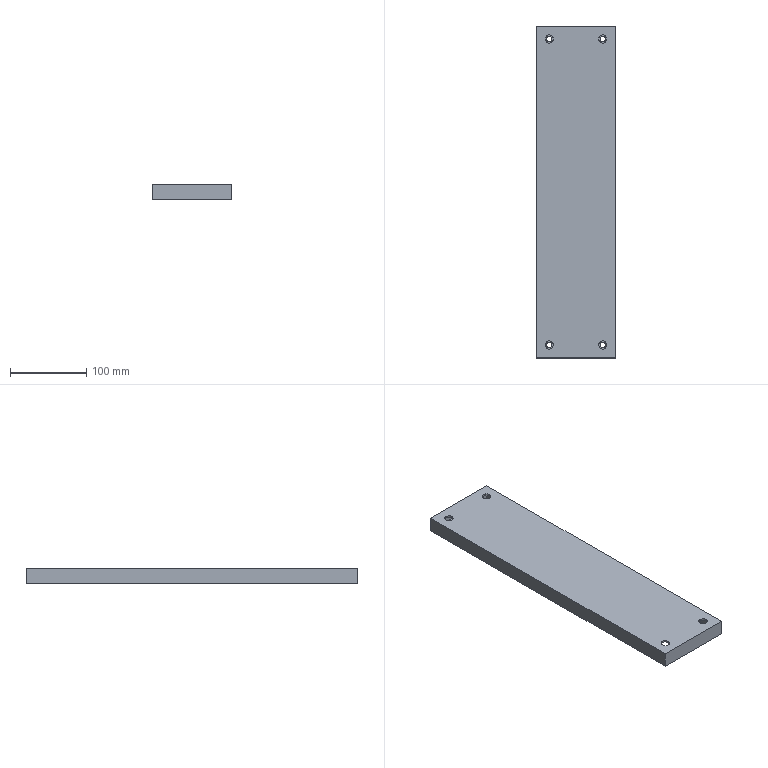Part | SolidWorks | features Extrusion 1, HoleWzd 1, ICE 1, Shell 1 | 1 solid | 32 faces | box 104 x 434 x 20 mm | volume 163254 mm3 | cylinder 16 | plane 16 | commonest cylinder face diameters 6.6 x8 11 x8
STEP:
#1=CARTESIAN_POINT('',(-29.5,200.,18.));
#2=VERTEX_POINT('',#1);
#3=CARTESIAN_POINT('',(-40.5,200.,18.));
#4=VERTEX_POINT('',#3);
#5=CARTESIAN_POINT('',(-35.,200.,18.));
#6=DIRECTION('',(0.,0.,-1.));
#7=DIRECTION('',(-1.,0.,0.));
#8=AXIS2_PLACEMENT_3D('',#5,#6,#7);
#9=CIRCLE('',#8,5.5);
#10=EDGE_CURVE('',#2,#4,#9,.T.);
#11=ORIENTED_EDGE('',*,*,#10,.T.);
#12=CARTESIAN_POINT('',(-40.5,200.,20.));
#13=VERTEX_POINT('',#12);
#14=CARTESIAN_POINT('',(-40.5,200.,20.));
#15=DIRECTION('',(0.,0.,1.));
#16=VECTOR('',#15,1000.);
#17=LINE('',#14,#16);
#18=EDGE_CURVE('',#4,#13,#17,.T.);
#19=ORIENTED_EDGE('',*,*,#18,.T.);
#20=CARTESIAN_POINT('',(-29.5,200.,20.));
#21=VERTEX_POINT('',#20);
#22=CARTESIAN_POINT('',(-35.,200.,20.));
#23=DIRECTION('',(0.,0.,1.));
#24=DIRECTION('',(1.,0.,0.));
#25=AXIS2_PLACEMENT_3D('',#22,#23,#24);
#26=CIRCLE('',#25,5.5);
#27=EDGE_CURVE('',#13,#21,#26,.T.);
#28=ORIENTED_EDGE('',*,*,#27,.T.);
#29=CARTESIAN_POINT('',(-29.5,200.,20.));
#30=DIRECTION('',(0.,0.,1.));
#31=VECTOR('',#30,1000.);
#32=LINE('',#29,#31);
#33=EDGE_CURVE('',#2,#21,#32,.T.);
#34=ORIENTED_EDGE('',*,*,#33,.F.);
#35=EDGE_LOOP('',(#11,#19,#28,#34));
#36=FACE_OUTER_BOUND('',#35,.T.);
#37=CARTESIAN_POINT('',(-35.,200.,20.));
#38=DIRECTION('',(0.,0.,1.));
#39=DIRECTION('',(1.,0.,0.));
#40=AXIS2_PLACEMENT_3D('',#37,#38,#39);
#41=CYLINDRICAL_SURFACE('',#40,5.5);
#42=ADVANCED_FACE('',(#36),#41,.F.);
#43=CARTESIAN_POINT('',(-38.3,200.,0.));
#44=VERTEX_POINT('',#43);
#45=CARTESIAN_POINT('',(-31.7,200.,0.));
#46=VERTEX_POINT('',#45);
#47=CARTESIAN_POINT('',(-35.,200.,0.));
#48=DIRECTION('',(0.,0.,1.));
#49=DIRECTION('',(1.,0.,0.));
#50=AXIS2_PLACEMENT_3D('',#47,#48,#49);
#51=CIRCLE('',#50,3.3);
#52=EDGE_CURVE('',#44,#46,#51,.T.);
#53=ORIENTED_EDGE('',*,*,#52,.F.);
#54=CARTESIAN_POINT('',(-38.3,200.,2.));
#55=VERTEX_POINT('',#54);
#56=CARTESIAN_POINT('',(-38.3,200.,20.));
#57=DIRECTION('',(0.,0.,1.));
#58=VECTOR('',#57,1000.);
#59=LINE('',#56,#58);
#60=EDGE_CURVE('',#44,#55,#59,.T.);
#61=ORIENTED_EDGE('',*,*,#60,.T.);
#62=CARTESIAN_POINT('',(-31.7,200.,2.));
#63=VERTEX_POINT('',#62);
#64=CARTESIAN_POINT('',(-35.,200.,2.));
#65=DIRECTION('',(0.,0.,-1.));
#66=DIRECTION('',(-1.,0.,0.));
#67=AXIS2_PLACEMENT_3D('',#64,#65,#66);
#68=CIRCLE('',#67,3.3);
#69=EDGE_CURVE('',#63,#55,#68,.T.);
#70=ORIENTED_EDGE('',*,*,#69,.F.);
#71=CARTESIAN_POINT('',(-31.7,200.,20.));
#72=DIRECTION('',(0.,0.,1.));
#73=VECTOR('',#72,1000.);
#74=LINE('',#71,#73);
#75=EDGE_CURVE('',#46,#63,#74,.T.);
#76=ORIENTED_EDGE('',*,*,#75,.F.);
#77=EDGE_LOOP('',(#53,#61,#70,#76));
#78=FACE_OUTER_BOUND('',#77,.T.);
#79=CARTESIAN_POINT('',(-35.,200.,20.));
#80=DIRECTION('',(0.,0.,1.));
#81=DIRECTION('',(1.,0.,0.));
#82=AXIS2_PLACEMENT_3D('',#79,#80,#81);
#83=CYLINDRICAL_SURFACE('',#82,3.3);
#84=ADVANCED_FACE('',(#78),#83,.F.);
#85=CARTESIAN_POINT('',(-29.5,-200.,18.));
#86=VERTEX_POINT('',#85);
#87=CARTESIAN_POINT('',(-40.5,-200.,18.));
#88=VERTEX_POINT('',#87);
#89=CARTESIAN_POINT('',(-35.,-200.,18.));
#90=DIRECTION('',(0.,0.,-1.));
#91=DIRECTION('',(-1.,0.,0.));
#92=AXIS2_PLACEMENT_3D('',#89,#90,#91);
#93=CIRCLE('',#92,5.5);
#94=EDGE_CURVE('',#86,#88,#93,.T.);
#95=ORIENTED_EDGE('',*,*,#94,.T.);
#96=CARTESIAN_POINT('',(-40.5,-200.,20.));
#97=VERTEX_POINT('',#96);
#98=CARTESIAN_POINT('',(-40.5,-200.,20.));
#99=DIRECTION('',(0.,0.,1.));
#100=VECTOR('',#99,1000.);
#101=LINE('',#98,#100);
#102=EDGE_CURVE('',#88,#97,#101,.T.);
#103=ORIENTED_EDGE('',*,*,#102,.T.);
#104=CARTESIAN_POINT('',(-29.5,-200.,20.));
#105=VERTEX_POINT('',#104);
#106=CARTESIAN_POINT('',(-35.,-200.,20.));
#107=DIRECTION('',(0.,0.,1.));
#108=DIRECTION('',(1.,0.,0.));
#109=AXIS2_PLACEMENT_3D('',#106,#107,#108);
#110=CIRCLE('',#109,5.5);
#111=EDGE_CURVE('',#97,#105,#110,.T.);
#112=ORIENTED_EDGE('',*,*,#111,.T.);
#113=CARTESIAN_POINT('',(-29.5,-200.,20.));
#114=DIRECTION('',(0.,0.,1.));
#115=VECTOR('',#114,1000.);
#116=LINE('',#113,#115);
#117=EDGE_CURVE('',#86,#105,#116,.T.);
#118=ORIENTED_EDGE('',*,*,#117,.F.);
#119=EDGE_LOOP('',(#95,#103,#112,#118));
#120=FACE_OUTER_BOUND('',#119,.T.);
#121=CARTESIAN_POINT('',(-35.,-200.,20.));
#122=DIRECTION('',(0.,0.,1.));
#123=DIRECTION('',(1.,0.,0.));
#124=AXIS2_PLACEMENT_3D('',#121,#122,#123);
#125=CYLINDRICAL_SURFACE('',#124,5.5);
#126=ADVANCED_FACE('',(#120),#125,.F.);
#127=CARTESIAN_POINT('',(-38.3,-200.,0.));
#128=VERTEX_POINT('',#127);
#129=CARTESIAN_POINT('',(-31.7,-200.,0.));
#130=VERTEX_POINT('',#129);
#131=CARTESIAN_POINT('',(-35.,-200.,0.));
#132=DIRECTION('',(0.,0.,1.));
#133=DIRECTION('',(1.,0.,0.));
#134=AXIS2_PLACEMENT_3D('',#131,#132,#133);
#135=CIRCLE('',#134,3.3);
#136=EDGE_CURVE('',#128,#130,#135,.T.);
#137=ORIENTED_EDGE('',*,*,#136,.F.);
#138=CARTESIAN_POINT('',(-38.3,-200.,2.));
#139=VERTEX_POINT('',#138);
#140=CARTESIAN_POINT('',(-38.3,-200.,20.));
#141=DIRECTION('',(0.,0.,1.));
#142=VECTOR('',#141,1000.);
#143=LINE('',#140,#142);
#144=EDGE_CURVE('',#128,#139,#143,.T.);
#145=ORIENTED_EDGE('',*,*,#144,.T.);
#146=CARTESIAN_POINT('',(-31.7,-200.,2.));
#147=VERTEX_POINT('',#146);
#148=CARTESIAN_POINT('',(-35.,-200.,2.));
#149=DIRECTION('',(0.,0.,-1.));
#150=DIRECTION('',(-1.,0.,0.));
#151=AXIS2_PLACEMENT_3D('',#148,#149,#150);
#152=CIRCLE('',#151,3.3);
#153=EDGE_CURVE('',#147,#139,#152,.T.);
#154=ORIENTED_EDGE('',*,*,#153,.F.);
#155=CARTESIAN_POINT('',(-31.7,-200.,20.));
#156=DIRECTION('',(0.,0.,1.));
#157=VECTOR('',#156,1000.);
#158=LINE('',#155,#157);
#159=EDGE_CURVE('',#130,#147,#158,.T.);
#160=ORIENTED_EDGE('',*,*,#159,.F.);
#161=EDGE_LOOP('',(#137,#145,#154,#160));
#162=FACE_OUTER_BOUND('',#161,.T.);
#163=CARTESIAN_POINT('',(-35.,-200.,20.));
#164=DIRECTION('',(0.,0.,1.));
#165=DIRECTION('',(1.,0.,0.));
#166=AXIS2_PLACEMENT_3D('',#163,#164,#165);
#167=CYLINDRICAL_SURFACE('',#166,3.3);
#168=ADVANCED_FACE('',(#162),#167,.F.);
#169=CARTESIAN_POINT('',(40.5,-200.,18.));
#170=VERTEX_POINT('',#169);
#171=CARTESIAN_POINT('',(29.5,-200.,18.));
#172=VERTEX_POINT('',#171);
#173=CARTESIAN_POINT('',(35.,-200.,18.));
#174=DIRECTION('',(0.,0.,-1.));
#175=DIRECTION('',(-1.,0.,0.));
#176=AXIS2_PLACEMENT_3D('',#173,#174,#175);
#177=CIRCLE('',#176,5.5);
#178=EDGE_CURVE('',#170,#172,#177,.T.);
#179=ORIENTED_EDGE('',*,*,#178,.T.);
#180=CARTESIAN_POINT('',(29.5,-200.,20.));
#181=VERTEX_POINT('',#180);
#182=CARTESIAN_POINT('',(29.5,-200.,20.));
#183=DIRECTION('',(0.,0.,1.));
#184=VECTOR('',#183,1000.);
#185=LINE('',#182,#184);
#186=EDGE_CURVE('',#172,#181,#185,.T.);
#187=ORIENTED_EDGE('',*,*,#186,.T.);
#188=CARTESIAN_POINT('',(40.5,-200.,20.));
#189=VERTEX_POINT('',#188);
#190=CARTESIAN_POINT('',(35.,-200.,20.));
#191=DIRECTION('',(0.,0.,1.));
#192=DIRECTION('',(1.,0.,0.));
#193=AXIS2_PLACEMENT_3D('',#190,#191,#192);
#194=CIRCLE('',#193,5.5);
#195=EDGE_CURVE('',#181,#189,#194,.T.);
#196=ORIENTED_EDGE('',*,*,#195,.T.);
#197=CARTESIAN_POINT('',(40.5,-200.,20.));
#198=DIRECTION('',(0.,0.,1.));
#199=VECTOR('',#198,1000.);
#200=LINE('',#197,#199);
#201=EDGE_CURVE('',#170,#189,#200,.T.);
#202=ORIENTED_EDGE('',*,*,#201,.F.);
#203=EDGE_LOOP('',(#179,#187,#196,#202));
#204=FACE_OUTER_BOUND('',#203,.T.);
#205=CARTESIAN_POINT('',(35.,-200.,20.));
#206=DIRECTION('',(0.,0.,1.));
#207=DIRECTION('',(1.,0.,0.));
#208=AXIS2_PLACEMENT_3D('',#205,#206,#207);
#209=CYLINDRICAL_SURFACE('',#208,5.5);
#210=ADVANCED_FACE('',(#204),#209,.F.);
#211=CARTESIAN_POINT('',(31.7,-200.,0.));
#212=VERTEX_POINT('',#211);
#213=CARTESIAN_POINT('',(38.3,-200.,0.));
#214=VERTEX_POINT('',#213);
#215=CARTESIAN_POINT('',(35.,-200.,0.));
#216=DIRECTION('',(0.,0.,1.));
#217=DIRECTION('',(1.,0.,0.));
#218=AXIS2_PLACEMENT_3D('',#215,#216,#217);
#219=CIRCLE('',#218,3.3);
#220=EDGE_CURVE('',#212,#214,#219,.T.);
#221=ORIENTED_EDGE('',*,*,#220,.F.);
#222=CARTESIAN_POINT('',(31.7,-200.,2.));
#223=VERTEX_POINT('',#222);
#224=CARTESIAN_POINT('',(31.7,-200.,20.));
#225=DIRECTION('',(0.,0.,1.));
#226=VECTOR('',#225,1000.);
#227=LINE('',#224,#226);
#228=EDGE_CURVE('',#212,#223,#227,.T.);
#229=ORIENTED_EDGE('',*,*,#228,.T.);
#230=CARTESIAN_POINT('',(38.3,-200.,2.));
#231=VERTEX_POINT('',#230);
#232=CARTESIAN_POINT('',(35.,-200.,2.));
#233=DIRECTION('',(0.,0.,-1.));
#234=DIRECTION('',(-1.,0.,0.));
#235=AXIS2_PLACEMENT_3D('',#232,#233,#234);
#236=CIRCLE('',#235,3.3);
#237=EDGE_CURVE('',#231,#223,#236,.T.);
#238=ORIENTED_EDGE('',*,*,#237,.F.);
#239=CARTESIAN_POINT('',(38.3,-200.,20.));
#240=DIRECTION('',(0.,0.,1.));
#241=VECTOR('',#240,1000.);
#242=LINE('',#239,#241);
#243=EDGE_CURVE('',#214,#231,#242,.T.);
#244=ORIENTED_EDGE('',*,*,#243,.F.);
#245=EDGE_LOOP('',(#221,#229,#238,#244));
#246=FACE_OUTER_BOUND('',#245,.T.);
#247=CARTESIAN_POINT('',(35.,-200.,20.));
#248=DIRECTION('',(0.,0.,1.));
#249=DIRECTION('',(1.,0.,0.));
#250=AXIS2_PLACEMENT_3D('',#247,#248,#249);
#251=CYLINDRICAL_SURFACE('',#250,3.3);
#252=ADVANCED_FACE('',(#246),#251,.F.);
#253=CARTESIAN_POINT('',(40.5,200.,18.));
#254=VERTEX_POINT('',#253);
#255=CARTESIAN_POINT('',(29.5,200.,18.));
#256=VERTEX_POINT('',#255);
#257=CARTESIAN_POINT('',(35.,200.,18.));
#258=DIRECTION('',(0.,0.,-1.));
#259=DIRECTION('',(-1.,0.,0.));
#260=AXIS2_PLACEMENT_3D('',#257,#258,#259);
#261=CIRCLE('',#260,5.5);
#262=EDGE_CURVE('',#254,#256,#261,.T.);
#263=ORIENTED_EDGE('',*,*,#262,.T.);
#264=CARTESIAN_POINT('',(29.5,200.,20.));
#265=VERTEX_POINT('',#264);
#266=CARTESIAN_POINT('',(29.5,200.,20.));
#267=DIRECTION('',(0.,0.,1.));
#268=VECTOR('',#267,1000.);
#269=LINE('',#266,#268);
#270=EDGE_CURVE('',#256,#265,#269,.T.);
#271=ORIENTED_EDGE('',*,*,#270,.T.);
#272=CARTESIAN_POINT('',(40.5,200.,20.));
#273=VERTEX_POINT('',#272);
#274=CARTESIAN_POINT('',(35.,200.,20.));
#275=DIRECTION('',(0.,0.,1.));
#276=DIRECTION('',(1.,0.,0.));
#277=AXIS2_PLACEMENT_3D('',#274,#275,#276);
#278=CIRCLE('',#277,5.5);
#279=EDGE_CURVE('',#265,#273,#278,.T.);
#280=ORIENTED_EDGE('',*,*,#279,.T.);
#281=CARTESIAN_POINT('',(40.5,200.,20.));
#282=DIRECTION('',(0.,0.,1.));
#283=VECTOR('',#282,1000.);
#284=LINE('',#281,#283);
#285=EDGE_CURVE('',#254,#273,#284,.T.);
#286=ORIENTED_EDGE('',*,*,#285,.F.);
#287=EDGE_LOOP('',(#263,#271,#280,#286));
#288=FACE_OUTER_BOUND('',#287,.T.);
#289=CARTESIAN_POINT('',(35.,200.,20.));
#290=DIRECTION('',(0.,0.,1.));
#291=DIRECTION('',(1.,0.,0.));
#292=AXIS2_PLACEMENT_3D('',#289,#290,#291);
#293=CYLINDRICAL_SURFACE('',#292,5.5);
#294=ADVANCED_FACE('',(#288),#293,.F.);
#295=CARTESIAN_POINT('',(31.7,200.,0.));
#296=VERTEX_POINT('',#295);
#297=CARTESIAN_POINT('',(38.3,200.,0.));
#298=VERTEX_POINT('',#297);
#299=CARTESIAN_POINT('',(35.,200.,0.));
#300=DIRECTION('',(0.,0.,1.));
#301=DIRECTION('',(1.,0.,0.));
#302=AXIS2_PLACEMENT_3D('',#299,#300,#301);
#303=CIRCLE('',#302,3.3);
#304=EDGE_CURVE('',#296,#298,#303,.T.);
#305=ORIENTED_EDGE('',*,*,#304,.F.);
#306=CARTESIAN_POINT('',(31.7,200.,2.));
#307=VERTEX_POINT('',#306);
#308=CARTESIAN_POINT('',(31.7,200.,20.));
#309=DIRECTION('',(0.,0.,1.));
#310=VECTOR('',#309,1000.);
#311=LINE('',#308,#310);
#312=EDGE_CURVE('',#296,#307,#311,.T.);
#313=ORIENTED_EDGE('',*,*,#312,.T.);
#314=CARTESIAN_POINT('',(38.3,200.,2.));
#315=VERTEX_POINT('',#314);
#316=CARTESIAN_POINT('',(35.,200.,2.));
#317=DIRECTION('',(0.,0.,-1.));
#318=DIRECTION('',(-1.,0.,0.));
#319=AXIS2_PLACEMENT_3D('',#316,#317,#318);
#320=CIRCLE('',#319,3.3);
#321=EDGE_CURVE('',#315,#307,#320,.T.);
#322=ORIENTED_EDGE('',*,*,#321,.F.);
#323=CARTESIAN_POINT('',(38.3,200.,20.));
#324=DIRECTION('',(0.,0.,1.));
#325=VECTOR('',#324,1000.);
#326=LINE('',#323,#325);
#327=EDGE_CURVE('',#298,#315,#326,.T.);
#328=ORIENTED_EDGE('',*,*,#327,.F.);
#329=EDGE_LOOP('',(#305,#313,#322,#328));
#330=FACE_OUTER_BOUND('',#329,.T.);
#331=CARTESIAN_POINT('',(35.,200.,20.));
#332=DIRECTION('',(0.,0.,1.));
#333=DIRECTION('',(1.,0.,0.));
#334=AXIS2_PLACEMENT_3D('',#331,#332,#333);
#335=CYLINDRICAL_SURFACE('',#334,3.3);
#336=ADVANCED_FACE('',(#330),#335,.F.);
#337=CARTESIAN_POINT('',(-35.,200.,0.));
#338=DIRECTION('',(0.,0.,1.));
#339=DIRECTION('',(1.,0.,0.));
#340=AXIS2_PLACEMENT_3D('',#337,#338,#339);
#341=CIRCLE('',#340,3.3);
#342=EDGE_CURVE('',#46,#44,#341,.T.);
#343=ORIENTED_EDGE('',*,*,#342,.T.);
#344=ORIENTED_EDGE('',*,*,#52,.T.);
#345=EDGE_LOOP('',(#343,#344));
#346=FACE_BOUND('',#345,.T.);
#347=CARTESIAN_POINT('',(-35.,-200.,0.));
#348=DIRECTION('',(0.,0.,1.));
#349=DIRECTION('',(1.,0.,0.));
#350=AXIS2_PLACEMENT_3D('',#347,#348,#349);
#351=CIRCLE('',#350,3.3);
#352=EDGE_CURVE('',#130,#128,#351,.T.);
#353=ORIENTED_EDGE('',*,*,#352,.T.);
#354=ORIENTED_EDGE('',*,*,#136,.T.);
#355=EDGE_LOOP('',(#353,#354));
#356=FACE_BOUND('',#355,.T.);
#357=CARTESIAN_POINT('',(35.,-200.,0.));
#358=DIRECTION('',(0.,0.,1.));
#359=DIRECTION('',(1.,0.,0.));
#360=AXIS2_PLACEMENT_3D('',#357,#358,#359);
#361=CIRCLE('',#360,3.3);
#362=EDGE_CURVE('',#214,#212,#361,.T.);
#363=ORIENTED_EDGE('',*,*,#362,.T.);
#364=ORIENTED_EDGE('',*,*,#220,.T.);
#365=EDGE_LOOP('',(#363,#364));
#366=FACE_BOUND('',#365,.T.);
#367=CARTESIAN_POINT('',(32.,-197.,0.));
#368=VERTEX_POINT('',#367);
#369=CARTESIAN_POINT('',(-32.,-197.,0.));
#370=VERTEX_POINT('',#369);
#371=CARTESIAN_POINT('',(32.,-197.,0.));
#372=DIRECTION('',(-1.,0.,0.));
#373=VECTOR('',#372,1000.);
#374=LINE('',#371,#373);
#375=EDGE_CURVE('',#368,#370,#374,.T.);
#376=ORIENTED_EDGE('',*,*,#375,.F.);
#377=CARTESIAN_POINT('',(32.,197.,0.));
#378=VERTEX_POINT('',#377);
#379=CARTESIAN_POINT('',(32.,-197.,0.));
#380=DIRECTION('',(0.,1.,0.));
#381=VECTOR('',#380,1000.);
#382=LINE('',#379,#381);
#383=EDGE_CURVE('',#368,#378,#382,.T.);
#384=ORIENTED_EDGE('',*,*,#383,.T.);
#385=CARTESIAN_POINT('',(-32.,197.,0.));
#386=VERTEX_POINT('',#385);
#387=CARTESIAN_POINT('',(32.,197.,0.));
#388=DIRECTION('',(-1.,0.,0.));
#389=VECTOR('',#388,1000.);
#390=LINE('',#387,#389);
#391=EDGE_CURVE('',#378,#386,#390,.T.);
#392=ORIENTED_EDGE('',*,*,#391,.T.);
#393=CARTESIAN_POINT('',(-32.,-197.,0.));
#394=DIRECTION('',(0.,1.,0.));
#395=VECTOR('',#394,1000.);
#396=LINE('',#393,#395);
#397=EDGE_CURVE('',#370,#386,#396,.T.);
#398=ORIENTED_EDGE('',*,*,#397,.F.);
#399=EDGE_LOOP('',(#376,#384,#392,#398));
#400=FACE_BOUND('',#399,.T.);
#401=CARTESIAN_POINT('',(52.,-217.,0.));
#402=VERTEX_POINT('',#401);
#403=CARTESIAN_POINT('',(52.,217.,0.));
#404=VERTEX_POINT('',#403);
#405=CARTESIAN_POINT('',(52.,-217.,0.));
#406=DIRECTION('',(0.,1.,0.));
#407=VECTOR('',#406,1000.);
#408=LINE('',#405,#407);
#409=EDGE_CURVE('',#402,#404,#408,.T.);
#410=ORIENTED_EDGE('',*,*,#409,.F.);
#411=CARTESIAN_POINT('',(-52.,-217.,0.));
#412=VERTEX_POINT('',#411);
#413=CARTESIAN_POINT('',(-52.,-217.,0.));
#414=DIRECTION('',(1.,0.,0.));
#415=VECTOR('',#414,1000.);
#416=LINE('',#413,#415);
#417=EDGE_CURVE('',#412,#402,#416,.T.);
#418=ORIENTED_EDGE('',*,*,#417,.F.);
#419=CARTESIAN_POINT('',(-52.,217.,0.));
#420=VERTEX_POINT('',#419);
#421=CARTESIAN_POINT('',(-52.,-217.,0.));
#422=DIRECTION('',(0.,-1.,0.));
#423=VECTOR('',#422,1000.);
#424=LINE('',#421,#423);
#425=EDGE_CURVE('',#420,#412,#424,.T.);
#426=ORIENTED_EDGE('',*,*,#425,.F.);
#427=CARTESIAN_POINT('',(-52.,217.,0.));
#428=DIRECTION('',(-1.,0.,0.));
#429=VECTOR('',#428,1000.);
#430=LINE('',#427,#429);
#431=EDGE_CURVE('',#404,#420,#430,.T.);
#432=ORIENTED_EDGE('',*,*,#431,.F.);
#433=EDGE_LOOP('',(#410,#418,#426,#432));
#434=FACE_OUTER_BOUND('',#433,.T.);
#435=CARTESIAN_POINT('',(35.,200.,0.));
#436=DIRECTION('',(0.,0.,1.));
#437=DIRECTION('',(1.,0.,0.));
#438=AXIS2_PLACEMENT_3D('',#435,#436,#437);
#439=CIRCLE('',#438,3.3);
#440=EDGE_CURVE('',#298,#296,#439,.T.);
#441=ORIENTED_EDGE('',*,*,#440,.T.);
#442=ORIENTED_EDGE('',*,*,#304,.T.);
#443=EDGE_LOOP('',(#441,#442));
#444=FACE_BOUND('',#443,.T.);
#445=CARTESIAN_POINT('',(0.,0.,0.));
#446=DIRECTION('',(0.,0.,-1.));
#447=DIRECTION('',(-1.,0.,0.));
#448=AXIS2_PLACEMENT_3D('',#445,#446,#447);
#449=PLANE('',#448);
#450=ADVANCED_FACE('',(#346,#356,#366,#400,#434,#444),#449,.T.);
#451=ORIENTED_EDGE('',*,*,#409,.T.);
#452=CARTESIAN_POINT('',(52.,217.,20.));
#453=VERTEX_POINT('',#452);
#454=CARTESIAN_POINT('',(52.,217.,20.));
#455=DIRECTION('',(0.,0.,-1.));
#456=VECTOR('',#455,1000.);
#457=LINE('',#454,#456);
#458=EDGE_CURVE('',#453,#404,#457,.T.);
#459=ORIENTED_EDGE('',*,*,#458,.F.);
#460=CARTESIAN_POINT('',(52.,-217.,20.));
#461=VERTEX_POINT('',#460);
#462=CARTESIAN_POINT('',(52.,-217.,20.));
#463=DIRECTION('',(0.,1.,0.));
#464=VECTOR('',#463,1000.);
#465=LINE('',#462,#464);
#466=EDGE_CURVE('',#461,#453,#465,.T.);
#467=ORIENTED_EDGE('',*,*,#466,.F.);
#468=CARTESIAN_POINT('',(52.,-217.,20.));
#469=DIRECTION('',(0.,0.,-1.));
#470=VECTOR('',#469,1000.);
#471=LINE('',#468,#470);
#472=EDGE_CURVE('',#461,#402,#471,.T.);
#473=ORIENTED_EDGE('',*,*,#472,.T.);
#474=EDGE_LOOP('',(#451,#459,#467,#473));
#475=FACE_OUTER_BOUND('',#474,.T.);
#476=CARTESIAN_POINT('',(52.,-217.,20.));
#477=DIRECTION('',(-1.,0.,0.));
#478=DIRECTION('',(0.,0.,1.));
#479=AXIS2_PLACEMENT_3D('',#476,#477,#478);
#480=PLANE('',#479);
#481=ADVANCED_FACE('',(#475),#480,.F.);
#482=ORIENTED_EDGE('',*,*,#431,.T.);
#483=CARTESIAN_POINT('',(-52.,217.,20.));
#484=VERTEX_POINT('',#483);
#485=CARTESIAN_POINT('',(-52.,217.,20.));
#486=DIRECTION('',(0.,0.,-1.));
#487=VECTOR('',#486,1000.);
#488=LINE('',#485,#487);
#489=EDGE_CURVE('',#484,#420,#488,.T.);
#490=ORIENTED_EDGE('',*,*,#489,.F.);
#491=CARTESIAN_POINT('',(-52.,217.,20.));
#492=DIRECTION('',(-1.,0.,0.));
#493=VECTOR('',#492,1000.);
#494=LINE('',#491,#493);
#495=EDGE_CURVE('',#453,#484,#494,.T.);
#496=ORIENTED_EDGE('',*,*,#495,.F.);
#497=ORIENTED_EDGE('',*,*,#458,.T.);
#498=EDGE_LOOP('',(#482,#490,#496,#497));
#499=FACE_OUTER_BOUND('',#498,.T.);
#500=CARTESIAN_POINT('',(-52.,217.,20.));
#501=DIRECTION('',(0.,-1.,0.));
#502=DIRECTION('',(0.,0.,-1.));
#503=AXIS2_PLACEMENT_3D('',#500,#501,#502);
#504=PLANE('',#503);
#505=ADVANCED_FACE('',(#499),#504,.F.);
#506=ORIENTED_EDGE('',*,*,#425,.T.);
#507=CARTESIAN_POINT('',(-52.,-217.,20.));
#508=VERTEX_POINT('',#507);
#509=CARTESIAN_POINT('',(-52.,-217.,20.));
#510=DIRECTION('',(0.,0.,-1.));
#511=VECTOR('',#510,1000.);
#512=LINE('',#509,#511);
#513=EDGE_CURVE('',#508,#412,#512,.T.);
#514=ORIENTED_EDGE('',*,*,#513,.F.);
#515=CARTESIAN_POINT('',(-52.,-217.,20.));
#516=DIRECTION('',(0.,-1.,0.));
#517=VECTOR('',#516,1000.);
#518=LINE('',#515,#517);
#519=EDGE_CURVE('',#484,#508,#518,.T.);
#520=ORIENTED_EDGE('',*,*,#519,.F.);
#521=ORIENTED_EDGE('',*,*,#489,.T.);
#522=EDGE_LOOP('',(#506,#514,#520,#521));
#523=FACE_OUTER_BOUND('',#522,.T.);
#524=CARTESIAN_POINT('',(-52.,-217.,20.));
#525=DIRECTION('',(1.,0.,0.));
#526=DIRECTION('',(0.,0.,-1.));
#527=AXIS2_PLACEMENT_3D('',#524,#525,#526);
#528=PLANE('',#527);
#529=ADVANCED_FACE('',(#523),#528,.F.);
#530=ORIENTED_EDGE('',*,*,#417,.T.);
#531=ORIENTED_EDGE('',*,*,#472,.F.);
#532=CARTESIAN_POINT('',(-52.,-217.,20.));
#533=DIRECTION('',(1.,0.,0.));
#534=VECTOR('',#533,1000.);
#535=LINE('',#532,#534);
#536=EDGE_CURVE('',#508,#461,#535,.T.);
#537=ORIENTED_EDGE('',*,*,#536,.F.);
#538=ORIENTED_EDGE('',*,*,#513,.T.);
#539=EDGE_LOOP('',(#530,#531,#537,#538));
#540=FACE_OUTER_BOUND('',#539,.T.);
#541=CARTESIAN_POINT('',(-52.,-217.,20.));
#542=DIRECTION('',(0.,1.,0.));
#543=DIRECTION('',(0.,0.,1.));
#544=AXIS2_PLACEMENT_3D('',#541,#542,#543);
#545=PLANE('',#544);
#546=ADVANCED_FACE('',(#540),#545,.F.);
#547=CARTESIAN_POINT('',(-35.,200.,20.));
#548=DIRECTION('',(0.,0.,1.));
#549=DIRECTION('',(1.,0.,0.));
#550=AXIS2_PLACEMENT_3D('',#547,#548,#549);
#551=CIRCLE('',#550,5.5);
#552=EDGE_CURVE('',#21,#13,#551,.T.);
#553=ORIENTED_EDGE('',*,*,#552,.F.);
#554=ORIENTED_EDGE('',*,*,#27,.F.);
#555=EDGE_LOOP('',(#553,#554));
#556=FACE_BOUND('',#555,.T.);
#557=CARTESIAN_POINT('',(-35.,-200.,20.));
#558=DIRECTION('',(0.,0.,1.));
#559=DIRECTION('',(1.,0.,0.));
#560=AXIS2_PLACEMENT_3D('',#557,#558,#559);
#561=CIRCLE('',#560,5.5);
#562=EDGE_CURVE('',#105,#97,#561,.T.);
#563=ORIENTED_EDGE('',*,*,#562,.F.);
#564=ORIENTED_EDGE('',*,*,#111,.F.);
#565=EDGE_LOOP('',(#563,#564));
#566=FACE_BOUND('',#565,.T.);
#567=CARTESIAN_POINT('',(35.,-200.,20.));
#568=DIRECTION('',(0.,0.,1.));
#569=DIRECTION('',(1.,0.,0.));
#570=AXIS2_PLACEMENT_3D('',#567,#568,#569);
#571=CIRCLE('',#570,5.5);
#572=EDGE_CURVE('',#189,#181,#571,.T.);
#573=ORIENTED_EDGE('',*,*,#572,.F.);
#574=ORIENTED_EDGE('',*,*,#195,.F.);
#575=EDGE_LOOP('',(#573,#574));
#576=FACE_BOUND('',#575,.T.);
#577=CARTESIAN_POINT('',(35.,200.,20.));
#578=DIRECTION('',(0.,0.,1.));
#579=DIRECTION('',(1.,0.,0.));
#580=AXIS2_PLACEMENT_3D('',#577,#578,#579);
#581=CIRCLE('',#580,5.5);
#582=EDGE_CURVE('',#273,#265,#581,.T.);
#583=ORIENTED_EDGE('',*,*,#582,.F.);
#584=ORIENTED_EDGE('',*,*,#279,.F.);
#585=EDGE_LOOP('',(#583,#584));
#586=FACE_BOUND('',#585,.T.);
#587=ORIENTED_EDGE('',*,*,#466,.T.);
#588=ORIENTED_EDGE('',*,*,#495,.T.);
#589=ORIENTED_EDGE('',*,*,#519,.T.);
#590=ORIENTED_EDGE('',*,*,#536,.T.);
#591=EDGE_LOOP('',(#587,#588,#589,#590));
#592=FACE_OUTER_BOUND('',#591,.T.);
#593=CARTESIAN_POINT('',(0.,0.,20.));
#594=DIRECTION('',(0.,0.,-1.));
#595=DIRECTION('',(-1.,0.,0.));
#596=AXIS2_PLACEMENT_3D('',#593,#594,#595);
#597=PLANE('',#596);
#598=ADVANCED_FACE('',(#556,#566,#576,#586,#592),#597,.F.);
#599=ORIENTED_EDGE('',*,*,#383,.F.);
#600=CARTESIAN_POINT('',(32.,-197.,2.));
#601=VERTEX_POINT('',#600);
#602=CARTESIAN_POINT('',(32.,-197.,2.));
#603=DIRECTION('',(0.,0.,-1.));
#604=VECTOR('',#603,1000.);
#605=LINE('',#602,#604);
#606=EDGE_CURVE('',#601,#368,#605,.T.);
#607=ORIENTED_EDGE('',*,*,#606,.F.);
#608=CARTESIAN_POINT('',(32.,197.,2.));
#609=VERTEX_POINT('',#608);
#610=CARTESIAN_POINT('',(32.,-197.,2.));
#611=DIRECTION('',(0.,1.,0.));
#612=VECTOR('',#611,1000.);
#613=LINE('',#610,#612);
#614=EDGE_CURVE('',#601,#609,#613,.T.);
#615=ORIENTED_EDGE('',*,*,#614,.T.);
#616=CARTESIAN_POINT('',(32.,197.,2.));
#617=DIRECTION('',(0.,0.,-1.));
#618=VECTOR('',#617,1000.);
#619=LINE('',#616,#618);
#620=EDGE_CURVE('',#609,#378,#619,.T.);
#621=ORIENTED_EDGE('',*,*,#620,.T.);
#622=EDGE_LOOP('',(#599,#607,#615,#621));
#623=FACE_OUTER_BOUND('',#622,.T.);
#624=CARTESIAN_POINT('',(32.,-197.,2.));
#625=DIRECTION('',(-1.,0.,0.));
#626=DIRECTION('',(0.,0.,1.));
#627=AXIS2_PLACEMENT_3D('',#624,#625,#626);
#628=PLANE('',#627);
#629=ADVANCED_FACE('',(#623),#628,.T.);
#630=ORIENTED_EDGE('',*,*,#391,.F.);
#631=ORIENTED_EDGE('',*,*,#620,.F.);
#632=CARTESIAN_POINT('',(-32.,197.,2.));
#633=VERTEX_POINT('',#632);
#634=CARTESIAN_POINT('',(32.,197.,2.));
#635=DIRECTION('',(-1.,0.,0.));
#636=VECTOR('',#635,1000.);
#637=LINE('',#634,#636);
#638=EDGE_CURVE('',#609,#633,#637,.T.);
#639=ORIENTED_EDGE('',*,*,#638,.T.);
#640=CARTESIAN_POINT('',(-32.,197.,2.));
#641=DIRECTION('',(0.,0.,-1.));
#642=VECTOR('',#641,1000.);
#643=LINE('',#640,#642);
#644=EDGE_CURVE('',#633,#386,#643,.T.);
#645=ORIENTED_EDGE('',*,*,#644,.T.);
#646=EDGE_LOOP('',(#630,#631,#639,#645));
#647=FACE_OUTER_BOUND('',#646,.T.);
#648=CARTESIAN_POINT('',(32.,197.,2.));
#649=DIRECTION('',(0.,-1.,0.));
#650=DIRECTION('',(0.,0.,-1.));
#651=AXIS2_PLACEMENT_3D('',#648,#649,#650);
#652=PLANE('',#651);
#653=ADVANCED_FACE('',(#647),#652,.T.);
#654=ORIENTED_EDGE('',*,*,#397,.T.);
#655=ORIENTED_EDGE('',*,*,#644,.F.);
#656=CARTESIAN_POINT('',(-32.,-197.,2.));
#657=VERTEX_POINT('',#656);
#658=CARTESIAN_POINT('',(-32.,-197.,2.));
#659=DIRECTION('',(0.,1.,0.));
#660=VECTOR('',#659,1000.);
#661=LINE('',#658,#660);
#662=EDGE_CURVE('',#657,#633,#661,.T.);
#663=ORIENTED_EDGE('',*,*,#662,.F.);
#664=CARTESIAN_POINT('',(-32.,-197.,2.));
#665=DIRECTION('',(0.,0.,-1.));
#666=VECTOR('',#665,1000.);
#667=LINE('',#664,#666);
#668=EDGE_CURVE('',#657,#370,#667,.T.);
#669=ORIENTED_EDGE('',*,*,#668,.T.);
#670=EDGE_LOOP('',(#654,#655,#663,#669));
#671=FACE_OUTER_BOUND('',#670,.T.);
#672=CARTESIAN_POINT('',(-32.,-197.,2.));
#673=DIRECTION('',(-1.,0.,0.));
#674=DIRECTION('',(0.,0.,1.));
#675=AXIS2_PLACEMENT_3D('',#672,#673,#674);
#676=PLANE('',#675);
#677=ADVANCED_FACE('',(#671),#676,.F.);
#678=ORIENTED_EDGE('',*,*,#375,.T.);
#679=ORIENTED_EDGE('',*,*,#668,.F.);
#680=CARTESIAN_POINT('',(32.,-197.,2.));
#681=DIRECTION('',(-1.,0.,0.));
#682=VECTOR('',#681,1000.);
#683=LINE('',#680,#682);
#684=EDGE_CURVE('',#601,#657,#683,.T.);
#685=ORIENTED_EDGE('',*,*,#684,.F.);
#686=ORIENTED_EDGE('',*,*,#606,.T.);
#687=EDGE_LOOP('',(#678,#679,#685,#686));
#688=FACE_OUTER_BOUND('',#687,.T.);
#689=CARTESIAN_POINT('',(32.,-197.,2.));
#690=DIRECTION('',(0.,-1.,0.));
#691=DIRECTION('',(0.,0.,-1.));
#692=AXIS2_PLACEMENT_3D('',#689,#690,#691);
#693=PLANE('',#692);
#694=ADVANCED_FACE('',(#688),#693,.F.);
#695=ORIENTED_EDGE('',*,*,#69,.T.);
#696=CARTESIAN_POINT('',(-35.,200.,2.));
#697=DIRECTION('',(0.,0.,-1.));
#698=DIRECTION('',(-1.,0.,0.));
#699=AXIS2_PLACEMENT_3D('',#696,#697,#698);
#700=CIRCLE('',#699,3.3);
#701=EDGE_CURVE('',#55,#63,#700,.T.);
#702=ORIENTED_EDGE('',*,*,#701,.T.);
#703=EDGE_LOOP('',(#695,#702));
#704=FACE_BOUND('',#703,.T.);
#705=ORIENTED_EDGE('',*,*,#153,.T.);
#706=CARTESIAN_POINT('',(-35.,-200.,2.));
#707=DIRECTION('',(0.,0.,-1.));
#708=DIRECTION('',(-1.,0.,0.));
#709=AXIS2_PLACEMENT_3D('',#706,#707,#708);
#710=CIRCLE('',#709,3.3);
#711=EDGE_CURVE('',#139,#147,#710,.T.);
#712=ORIENTED_EDGE('',*,*,#711,.T.);
#713=EDGE_LOOP('',(#705,#712));
#714=FACE_BOUND('',#713,.T.);
#715=ORIENTED_EDGE('',*,*,#237,.T.);
#716=CARTESIAN_POINT('',(35.,-200.,2.));
#717=DIRECTION('',(0.,0.,-1.));
#718=DIRECTION('',(-1.,0.,0.));
#719=AXIS2_PLACEMENT_3D('',#716,#717,#718);
#720=CIRCLE('',#719,3.3);
#721=EDGE_CURVE('',#223,#231,#720,.T.);
#722=ORIENTED_EDGE('',*,*,#721,.T.);
#723=EDGE_LOOP('',(#715,#722));
#724=FACE_BOUND('',#723,.T.);
#725=ORIENTED_EDGE('',*,*,#321,.T.);
#726=CARTESIAN_POINT('',(35.,200.,2.));
#727=DIRECTION('',(0.,0.,-1.));
#728=DIRECTION('',(-1.,0.,0.));
#729=AXIS2_PLACEMENT_3D('',#726,#727,#728);
#730=CIRCLE('',#729,3.3);
#731=EDGE_CURVE('',#307,#315,#730,.T.);
#732=ORIENTED_EDGE('',*,*,#731,.T.);
#733=EDGE_LOOP('',(#725,#732));
#734=FACE_BOUND('',#733,.T.);
#735=CARTESIAN_POINT('',(50.,-215.,2.));
#736=VERTEX_POINT('',#735);
#737=CARTESIAN_POINT('',(50.,215.,2.));
#738=VERTEX_POINT('',#737);
#739=CARTESIAN_POINT('',(50.,0.,2.));
#740=DIRECTION('',(0.,1.,0.));
#741=VECTOR('',#740,1000.);
#742=LINE('',#739,#741);
#743=EDGE_CURVE('',#736,#738,#742,.T.);
#744=ORIENTED_EDGE('',*,*,#743,.T.);
#745=CARTESIAN_POINT('',(-50.,215.,2.));
#746=VERTEX_POINT('',#745);
#747=CARTESIAN_POINT('',(0.,215.,2.));
#748=DIRECTION('',(-1.,0.,0.));
#749=VECTOR('',#748,1000.);
#750=LINE('',#747,#749);
#751=EDGE_CURVE('',#738,#746,#750,.T.);
#752=ORIENTED_EDGE('',*,*,#751,.T.);
#753=CARTESIAN_POINT('',(-50.,-215.,2.));
#754=VERTEX_POINT('',#753);
#755=CARTESIAN_POINT('',(-50.,0.,2.));
#756=DIRECTION('',(0.,-1.,0.));
#757=VECTOR('',#756,1000.);
#758=LINE('',#755,#757);
#759=EDGE_CURVE('',#746,#754,#758,.T.);
#760=ORIENTED_EDGE('',*,*,#759,.T.);
#761=CARTESIAN_POINT('',(0.,-215.,2.));
#762=DIRECTION('',(1.,0.,0.));
#763=VECTOR('',#762,1000.);
#764=LINE('',#761,#763);
#765=EDGE_CURVE('',#754,#736,#764,.T.);
#766=ORIENTED_EDGE('',*,*,#765,.T.);
#767=EDGE_LOOP('',(#744,#752,#760,#766));
#768=FACE_OUTER_BOUND('',#767,.T.);
#769=ORIENTED_EDGE('',*,*,#684,.T.);
#770=ORIENTED_EDGE('',*,*,#662,.T.);
#771=ORIENTED_EDGE('',*,*,#638,.F.);
#772=ORIENTED_EDGE('',*,*,#614,.F.);
#773=EDGE_LOOP('',(#769,#770,#771,#772));
#774=FACE_BOUND('',#773,.T.);
#775=CARTESIAN_POINT('',(0.,0.,2.));
#776=DIRECTION('',(0.,0.,-1.));
#777=DIRECTION('',(-1.,0.,0.));
#778=AXIS2_PLACEMENT_3D('',#775,#776,#777);
#779=PLANE('',#778);
#780=ADVANCED_FACE('',(#704,#714,#724,#734,#768,#774),#779,.F.);
#781=ORIENTED_EDGE('',*,*,#743,.F.);
#782=CARTESIAN_POINT('',(50.,-215.,18.));
#783=VERTEX_POINT('',#782);
#784=CARTESIAN_POINT('',(50.,-215.,20.));
#785=DIRECTION('',(0.,0.,-1.));
#786=VECTOR('',#785,1000.);
#787=LINE('',#784,#786);
#788=EDGE_CURVE('',#783,#736,#787,.T.);
#789=ORIENTED_EDGE('',*,*,#788,.F.);
#790=CARTESIAN_POINT('',(50.,215.,18.));
#791=VERTEX_POINT('',#790);
#792=CARTESIAN_POINT('',(50.,0.,18.));
#793=DIRECTION('',(0.,1.,0.));
#794=VECTOR('',#793,1000.);
#795=LINE('',#792,#794);
#796=EDGE_CURVE('',#783,#791,#795,.T.);
#797=ORIENTED_EDGE('',*,*,#796,.T.);
#798=CARTESIAN_POINT('',(50.,215.,20.));
#799=DIRECTION('',(0.,0.,-1.));
#800=VECTOR('',#799,1000.);
#801=LINE('',#798,#800);
#802=EDGE_CURVE('',#791,#738,#801,.T.);
#803=ORIENTED_EDGE('',*,*,#802,.T.);
#804=EDGE_LOOP('',(#781,#789,#797,#803));
#805=FACE_OUTER_BOUND('',#804,.T.);
#806=CARTESIAN_POINT('',(50.,-217.,20.));
#807=DIRECTION('',(-1.,0.,0.));
#808=DIRECTION('',(0.,0.,1.));
#809=AXIS2_PLACEMENT_3D('',#806,#807,#808);
#810=PLANE('',#809);
#811=ADVANCED_FACE('',(#805),#810,.T.);
#812=ORIENTED_EDGE('',*,*,#751,.F.);
#813=ORIENTED_EDGE('',*,*,#802,.F.);
#814=CARTESIAN_POINT('',(-50.,215.,18.));
#815=VERTEX_POINT('',#814);
#816=CARTESIAN_POINT('',(0.,215.,18.));
#817=DIRECTION('',(-1.,0.,0.));
#818=VECTOR('',#817,1000.);
#819=LINE('',#816,#818);
#820=EDGE_CURVE('',#791,#815,#819,.T.);
#821=ORIENTED_EDGE('',*,*,#820,.T.);
#822=CARTESIAN_POINT('',(-50.,215.,20.));
#823=DIRECTION('',(0.,0.,-1.));
#824=VECTOR('',#823,1000.);
#825=LINE('',#822,#824);
#826=EDGE_CURVE('',#815,#746,#825,.T.);
#827=ORIENTED_EDGE('',*,*,#826,.T.);
#828=EDGE_LOOP('',(#812,#813,#821,#827));
#829=FACE_OUTER_BOUND('',#828,.T.);
#830=CARTESIAN_POINT('',(-52.,215.,20.));
#831=DIRECTION('',(0.,-1.,0.));
#832=DIRECTION('',(0.,0.,-1.));
#833=AXIS2_PLACEMENT_3D('',#830,#831,#832);
#834=PLANE('',#833);
#835=ADVANCED_FACE('',(#829),#834,.T.);
#836=ORIENTED_EDGE('',*,*,#759,.F.);
#837=ORIENTED_EDGE('',*,*,#826,.F.);
#838=CARTESIAN_POINT('',(-50.,-215.,18.));
#839=VERTEX_POINT('',#838);
#840=CARTESIAN_POINT('',(-50.,0.,18.));
#841=DIRECTION('',(0.,-1.,0.));
#842=VECTOR('',#841,1000.);
#843=LINE('',#840,#842);
#844=EDGE_CURVE('',#815,#839,#843,.T.);
#845=ORIENTED_EDGE('',*,*,#844,.T.);
#846=CARTESIAN_POINT('',(-50.,-215.,20.));
#847=DIRECTION('',(0.,0.,-1.));
#848=VECTOR('',#847,1000.);
#849=LINE('',#846,#848);
#850=EDGE_CURVE('',#839,#754,#849,.T.);
#851=ORIENTED_EDGE('',*,*,#850,.T.);
#852=EDGE_LOOP('',(#836,#837,#845,#851));
#853=FACE_OUTER_BOUND('',#852,.T.);
#854=CARTESIAN_POINT('',(-50.,-217.,20.));
#855=DIRECTION('',(1.,0.,0.));
#856=DIRECTION('',(0.,0.,-1.));
#857=AXIS2_PLACEMENT_3D('',#854,#855,#856);
#858=PLANE('',#857);
#859=ADVANCED_FACE('',(#853),#858,.T.);
#860=ORIENTED_EDGE('',*,*,#765,.F.);
#861=ORIENTED_EDGE('',*,*,#850,.F.);
#862=CARTESIAN_POINT('',(0.,-215.,18.));
#863=DIRECTION('',(1.,0.,0.));
#864=VECTOR('',#863,1000.);
#865=LINE('',#862,#864);
#866=EDGE_CURVE('',#839,#783,#865,.T.);
#867=ORIENTED_EDGE('',*,*,#866,.T.);
#868=ORIENTED_EDGE('',*,*,#788,.T.);
#869=EDGE_LOOP('',(#860,#861,#867,#868));
#870=FACE_OUTER_BOUND('',#869,.T.);
#871=CARTESIAN_POINT('',(-52.,-215.,20.));
#872=DIRECTION('',(0.,1.,0.));
#873=DIRECTION('',(0.,0.,1.));
#874=AXIS2_PLACEMENT_3D('',#871,#872,#873);
#875=PLANE('',#874);
#876=ADVANCED_FACE('',(#870),#875,.T.);
#877=ORIENTED_EDGE('',*,*,#10,.F.);
#878=CARTESIAN_POINT('',(-35.,200.,18.));
#879=DIRECTION('',(0.,0.,-1.));
#880=DIRECTION('',(-1.,0.,0.));
#881=AXIS2_PLACEMENT_3D('',#878,#879,#880);
#882=CIRCLE('',#881,5.5);
#883=EDGE_CURVE('',#4,#2,#882,.T.);
#884=ORIENTED_EDGE('',*,*,#883,.F.);
#885=EDGE_LOOP('',(#877,#884));
#886=FACE_BOUND('',#885,.T.);
#887=ORIENTED_EDGE('',*,*,#94,.F.);
#888=CARTESIAN_POINT('',(-35.,-200.,18.));
#889=DIRECTION('',(0.,0.,-1.));
#890=DIRECTION('',(-1.,0.,0.));
#891=AXIS2_PLACEMENT_3D('',#888,#889,#890);
#892=CIRCLE('',#891,5.5);
#893=EDGE_CURVE('',#88,#86,#892,.T.);
#894=ORIENTED_EDGE('',*,*,#893,.F.);
#895=EDGE_LOOP('',(#887,#894));
#896=FACE_BOUND('',#895,.T.);
#897=ORIENTED_EDGE('',*,*,#178,.F.);
#898=CARTESIAN_POINT('',(35.,-200.,18.));
#899=DIRECTION('',(0.,0.,-1.));
#900=DIRECTION('',(-1.,0.,0.));
#901=AXIS2_PLACEMENT_3D('',#898,#899,#900);
#902=CIRCLE('',#901,5.5);
#903=EDGE_CURVE('',#172,#170,#902,.T.);
#904=ORIENTED_EDGE('',*,*,#903,.F.);
#905=EDGE_LOOP('',(#897,#904));
#906=FACE_BOUND('',#905,.T.);
#907=ORIENTED_EDGE('',*,*,#262,.F.);
#908=CARTESIAN_POINT('',(35.,200.,18.));
#909=DIRECTION('',(0.,0.,-1.));
#910=DIRECTION('',(-1.,0.,0.));
#911=AXIS2_PLACEMENT_3D('',#908,#909,#910);
#912=CIRCLE('',#911,5.5);
#913=EDGE_CURVE('',#256,#254,#912,.T.);
#914=ORIENTED_EDGE('',*,*,#913,.F.);
#915=EDGE_LOOP('',(#907,#914));
#916=FACE_BOUND('',#915,.T.);
#917=ORIENTED_EDGE('',*,*,#796,.F.);
#918=ORIENTED_EDGE('',*,*,#866,.F.);
#919=ORIENTED_EDGE('',*,*,#844,.F.);
#920=ORIENTED_EDGE('',*,*,#820,.F.);
#921=EDGE_LOOP('',(#917,#918,#919,#920));
#922=FACE_OUTER_BOUND('',#921,.T.);
#923=CARTESIAN_POINT('',(0.,0.,18.));
#924=DIRECTION('',(0.,0.,-1.));
#925=DIRECTION('',(-1.,0.,0.));
#926=AXIS2_PLACEMENT_3D('',#923,#924,#925);
#927=PLANE('',#926);
#928=ADVANCED_FACE('',(#886,#896,#906,#916,#922),#927,.T.);
#929=ORIENTED_EDGE('',*,*,#312,.F.);
#930=ORIENTED_EDGE('',*,*,#440,.F.);
#931=ORIENTED_EDGE('',*,*,#327,.T.);
#932=ORIENTED_EDGE('',*,*,#731,.F.);
#933=EDGE_LOOP('',(#929,#930,#931,#932));
#934=FACE_OUTER_BOUND('',#933,.T.);
#935=CARTESIAN_POINT('',(35.,200.,20.));
#936=DIRECTION('',(0.,0.,1.));
#937=DIRECTION('',(1.,0.,0.));
#938=AXIS2_PLACEMENT_3D('',#935,#936,#937);
#939=CYLINDRICAL_SURFACE('',#938,3.3);
#940=ADVANCED_FACE('',(#934),#939,.F.);
#941=ORIENTED_EDGE('',*,*,#270,.F.);
#942=ORIENTED_EDGE('',*,*,#913,.T.);
#943=ORIENTED_EDGE('',*,*,#285,.T.);
#944=ORIENTED_EDGE('',*,*,#582,.T.);
#945=EDGE_LOOP('',(#941,#942,#943,#944));
#946=FACE_OUTER_BOUND('',#945,.T.);
#947=CARTESIAN_POINT('',(35.,200.,20.));
#948=DIRECTION('',(0.,0.,1.));
#949=DIRECTION('',(1.,0.,0.));
#950=AXIS2_PLACEMENT_3D('',#947,#948,#949);
#951=CYLINDRICAL_SURFACE('',#950,5.5);
#952=ADVANCED_FACE('',(#946),#951,.F.);
#953=ORIENTED_EDGE('',*,*,#228,.F.);
#954=ORIENTED_EDGE('',*,*,#362,.F.);
#955=ORIENTED_EDGE('',*,*,#243,.T.);
#956=ORIENTED_EDGE('',*,*,#721,.F.);
#957=EDGE_LOOP('',(#953,#954,#955,#956));
#958=FACE_OUTER_BOUND('',#957,.T.);
#959=CARTESIAN_POINT('',(35.,-200.,20.));
#960=DIRECTION('',(0.,0.,1.));
#961=DIRECTION('',(1.,0.,0.));
#962=AXIS2_PLACEMENT_3D('',#959,#960,#961);
#963=CYLINDRICAL_SURFACE('',#962,3.3);
#964=ADVANCED_FACE('',(#958),#963,.F.);
#965=ORIENTED_EDGE('',*,*,#186,.F.);
#966=ORIENTED_EDGE('',*,*,#903,.T.);
#967=ORIENTED_EDGE('',*,*,#201,.T.);
#968=ORIENTED_EDGE('',*,*,#572,.T.);
#969=EDGE_LOOP('',(#965,#966,#967,#968));
#970=FACE_OUTER_BOUND('',#969,.T.);
#971=CARTESIAN_POINT('',(35.,-200.,20.));
#972=DIRECTION('',(0.,0.,1.));
#973=DIRECTION('',(1.,0.,0.));
#974=AXIS2_PLACEMENT_3D('',#971,#972,#973);
#975=CYLINDRICAL_SURFACE('',#974,5.5);
#976=ADVANCED_FACE('',(#970),#975,.F.);
#977=ORIENTED_EDGE('',*,*,#144,.F.);
#978=ORIENTED_EDGE('',*,*,#352,.F.);
#979=ORIENTED_EDGE('',*,*,#159,.T.);
#980=ORIENTED_EDGE('',*,*,#711,.F.);
#981=EDGE_LOOP('',(#977,#978,#979,#980));
#982=FACE_OUTER_BOUND('',#981,.T.);
#983=CARTESIAN_POINT('',(-35.,-200.,20.));
#984=DIRECTION('',(0.,0.,1.));
#985=DIRECTION('',(1.,0.,0.));
#986=AXIS2_PLACEMENT_3D('',#983,#984,#985);
#987=CYLINDRICAL_SURFACE('',#986,3.3);
#988=ADVANCED_FACE('',(#982),#987,.F.);
#989=ORIENTED_EDGE('',*,*,#102,.F.);
#990=ORIENTED_EDGE('',*,*,#893,.T.);
#991=ORIENTED_EDGE('',*,*,#117,.T.);
#992=ORIENTED_EDGE('',*,*,#562,.T.);
#993=EDGE_LOOP('',(#989,#990,#991,#992));
#994=FACE_OUTER_BOUND('',#993,.T.);
#995=CARTESIAN_POINT('',(-35.,-200.,20.));
#996=DIRECTION('',(0.,0.,1.));
#997=DIRECTION('',(1.,0.,0.));
#998=AXIS2_PLACEMENT_3D('',#995,#996,#997);
#999=CYLINDRICAL_SURFACE('',#998,5.5);
#1000=ADVANCED_FACE('',(#994),#999,.F.);
#1001=ORIENTED_EDGE('',*,*,#60,.F.);
#1002=ORIENTED_EDGE('',*,*,#342,.F.);
#1003=ORIENTED_EDGE('',*,*,#75,.T.);
#1004=ORIENTED_EDGE('',*,*,#701,.F.);
#1005=EDGE_LOOP('',(#1001,#1002,#1003,#1004));
#1006=FACE_OUTER_BOUND('',#1005,.T.);
#1007=CARTESIAN_POINT('',(-35.,200.,20.));
#1008=DIRECTION('',(0.,0.,1.));
#1009=DIRECTION('',(1.,0.,0.));
#1010=AXIS2_PLACEMENT_3D('',#1007,#1008,#1009);
#1011=CYLINDRICAL_SURFACE('',#1010,3.3);
#1012=ADVANCED_FACE('',(#1006),#1011,.F.);
#1013=ORIENTED_EDGE('',*,*,#18,.F.);
#1014=ORIENTED_EDGE('',*,*,#883,.T.);
#1015=ORIENTED_EDGE('',*,*,#33,.T.);
#1016=ORIENTED_EDGE('',*,*,#552,.T.);
#1017=EDGE_LOOP('',(#1013,#1014,#1015,#1016));
#1018=FACE_OUTER_BOUND('',#1017,.T.);
#1019=CARTESIAN_POINT('',(-35.,200.,20.));
#1020=DIRECTION('',(0.,0.,1.));
#1021=DIRECTION('',(1.,0.,0.));
#1022=AXIS2_PLACEMENT_3D('',#1019,#1020,#1021);
#1023=CYLINDRICAL_SURFACE('',#1022,5.5);
#1024=ADVANCED_FACE('',(#1018),#1023,.F.);
#1025=CLOSED_SHELL('',(#42,#84,#126,#168,#210,#252,#294,#336,#450,#481,#505,#529,#546,#598,#629,#653,#677,#694,#780,#811,#835,#859,#876,#928,#940,#952,#964,#976,#988,#1000,#1012,#1024));
#1026=MANIFOLD_SOLID_BREP('',#1025);
#1027=CARTESIAN_POINT('',(0.,0.,0.));
#1028=DIRECTION('',(0.,0.,1.));
#1029=DIRECTION('',(1.,0.,0.));
#1030=AXIS2_PLACEMENT_3D('',#1027,#1028,#1029);
#1031=(LENGTH_UNIT()NAMED_UNIT(*)SI_UNIT(.MILLI.,.METRE.));
#1032=UNCERTAINTY_MEASURE_WITH_UNIT(LENGTH_MEASURE(0.00001),#1031,'','');
#1033=(NAMED_UNIT(*)PLANE_ANGLE_UNIT()SI_UNIT($,.RADIAN.));
#1034=(NAMED_UNIT(*)SI_UNIT($,.STERADIAN.)SOLID_ANGLE_UNIT());
#1035=(GEOMETRIC_REPRESENTATION_CONTEXT(3)GLOBAL_UNCERTAINTY_ASSIGNED_CONTEXT((#1032))GLOBAL_UNIT_ASSIGNED_CONTEXT((#1031,#1033,#1034))REPRESENTATION_CONTEXT('',''));
#1036=ADVANCED_BREP_SHAPE_REPRESENTATION('',(#1026,#1030),#1035);